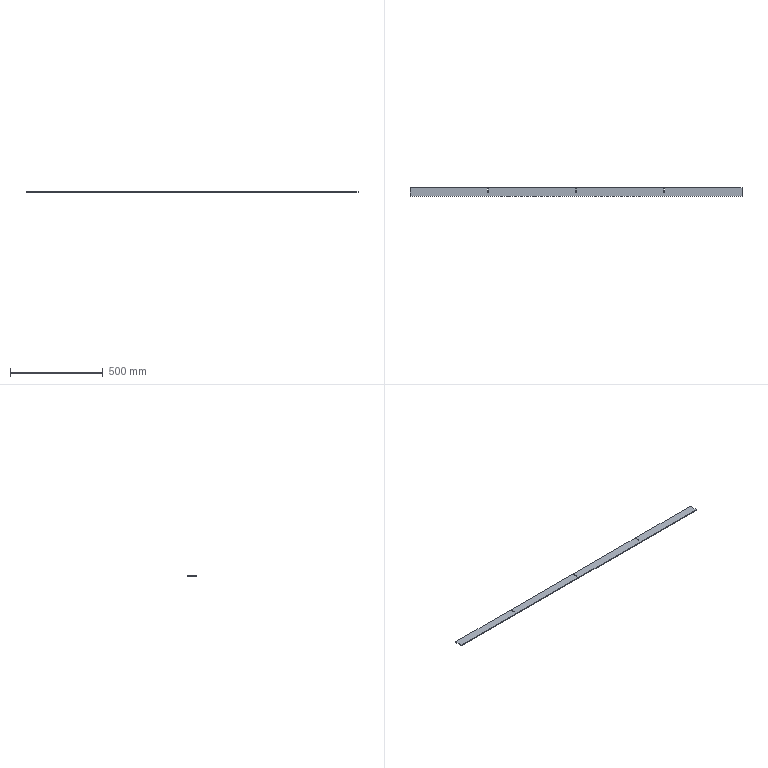Part | SolidWorks | features FlatPattern 1, SMBaseFlange 1, SheetMetal 1 | 1 solid | 18 faces | box 1790 x 45 x 4.5 mm | volume 360956 mm3 | plane 18
STEP:
#1=CARTESIAN_POINT('',(895.,-22.5,0.));
#2=VERTEX_POINT('',#1);
#3=CARTESIAN_POINT('',(895.,22.5,0.));
#4=VERTEX_POINT('',#3);
#5=CARTESIAN_POINT('',(895.,22.5,0.));
#6=DIRECTION('',(0.,1.,0.));
#7=VECTOR('',#6,1000.);
#8=LINE('',#5,#7);
#9=EDGE_CURVE('',#2,#4,#8,.T.);
#10=ORIENTED_EDGE('',*,*,#9,.F.);
#11=CARTESIAN_POINT('',(895.,-22.5,-4.5));
#12=VERTEX_POINT('',#11);
#13=CARTESIAN_POINT('',(895.,-22.5,-4.5));
#14=DIRECTION('',(0.,0.,1.));
#15=VECTOR('',#14,1000.);
#16=LINE('',#13,#15);
#17=EDGE_CURVE('',#12,#2,#16,.T.);
#18=ORIENTED_EDGE('',*,*,#17,.F.);
#19=CARTESIAN_POINT('',(895.,22.5,-4.5));
#20=VERTEX_POINT('',#19);
#21=CARTESIAN_POINT('',(895.,22.5,-4.5));
#22=DIRECTION('',(0.,1.,0.));
#23=VECTOR('',#22,1000.);
#24=LINE('',#21,#23);
#25=EDGE_CURVE('',#12,#20,#24,.T.);
#26=ORIENTED_EDGE('',*,*,#25,.T.);
#27=CARTESIAN_POINT('',(895.,22.5,-4.5));
#28=DIRECTION('',(0.,0.,1.));
#29=VECTOR('',#28,1000.);
#30=LINE('',#27,#29);
#31=EDGE_CURVE('',#20,#4,#30,.T.);
#32=ORIENTED_EDGE('',*,*,#31,.T.);
#33=EDGE_LOOP('',(#10,#18,#26,#32));
#34=FACE_OUTER_BOUND('',#33,.T.);
#35=CARTESIAN_POINT('',(895.,22.5,-4.5));
#36=DIRECTION('',(1.,0.,0.));
#37=DIRECTION('',(0.,0.,-1.));
#38=AXIS2_PLACEMENT_3D('',#35,#36,#37);
#39=PLANE('',#38);
#40=ADVANCED_FACE('',(#34),#39,.T.);
#41=CARTESIAN_POINT('',(-895.,-22.5,0.));
#42=VERTEX_POINT('',#41);
#43=CARTESIAN_POINT('',(-895.,-22.5,0.));
#44=DIRECTION('',(1.,0.,0.));
#45=VECTOR('',#44,1000.);
#46=LINE('',#43,#45);
#47=EDGE_CURVE('',#42,#2,#46,.T.);
#48=ORIENTED_EDGE('',*,*,#47,.F.);
#49=CARTESIAN_POINT('',(-895.,-22.5,-4.5));
#50=VERTEX_POINT('',#49);
#51=CARTESIAN_POINT('',(-895.,-22.5,-4.5));
#52=DIRECTION('',(0.,0.,1.));
#53=VECTOR('',#52,1000.);
#54=LINE('',#51,#53);
#55=EDGE_CURVE('',#50,#42,#54,.T.);
#56=ORIENTED_EDGE('',*,*,#55,.F.);
#57=CARTESIAN_POINT('',(-895.,-22.5,-4.5));
#58=DIRECTION('',(1.,0.,0.));
#59=VECTOR('',#58,1000.);
#60=LINE('',#57,#59);
#61=EDGE_CURVE('',#50,#12,#60,.T.);
#62=ORIENTED_EDGE('',*,*,#61,.T.);
#63=ORIENTED_EDGE('',*,*,#17,.T.);
#64=EDGE_LOOP('',(#48,#56,#62,#63));
#65=FACE_OUTER_BOUND('',#64,.T.);
#66=CARTESIAN_POINT('',(-895.,-22.5,-4.5));
#67=DIRECTION('',(0.,-1.,0.));
#68=DIRECTION('',(0.,0.,-1.));
#69=AXIS2_PLACEMENT_3D('',#66,#67,#68);
#70=PLANE('',#69);
#71=ADVANCED_FACE('',(#65),#70,.T.);
#72=CARTESIAN_POINT('',(-895.,22.5,0.));
#73=VERTEX_POINT('',#72);
#74=CARTESIAN_POINT('',(-895.,22.5,0.));
#75=DIRECTION('',(0.,-1.,0.));
#76=VECTOR('',#75,1000.);
#77=LINE('',#74,#76);
#78=EDGE_CURVE('',#73,#42,#77,.T.);
#79=ORIENTED_EDGE('',*,*,#78,.F.);
#80=CARTESIAN_POINT('',(-895.,22.5,-4.5));
#81=VERTEX_POINT('',#80);
#82=CARTESIAN_POINT('',(-895.,22.5,-4.5));
#83=DIRECTION('',(0.,0.,1.));
#84=VECTOR('',#83,1000.);
#85=LINE('',#82,#84);
#86=EDGE_CURVE('',#81,#73,#85,.T.);
#87=ORIENTED_EDGE('',*,*,#86,.F.);
#88=CARTESIAN_POINT('',(-895.,22.5,-4.5));
#89=DIRECTION('',(0.,-1.,0.));
#90=VECTOR('',#89,1000.);
#91=LINE('',#88,#90);
#92=EDGE_CURVE('',#81,#50,#91,.T.);
#93=ORIENTED_EDGE('',*,*,#92,.T.);
#94=ORIENTED_EDGE('',*,*,#55,.T.);
#95=EDGE_LOOP('',(#79,#87,#93,#94));
#96=FACE_OUTER_BOUND('',#95,.T.);
#97=CARTESIAN_POINT('',(-895.,22.5,-4.5));
#98=DIRECTION('',(-1.,0.,0.));
#99=DIRECTION('',(0.,0.,1.));
#100=AXIS2_PLACEMENT_3D('',#97,#98,#99);
#101=PLANE('',#100);
#102=ADVANCED_FACE('',(#96),#101,.T.);
#103=CARTESIAN_POINT('',(-477.25,22.5,0.));
#104=VERTEX_POINT('',#103);
#105=CARTESIAN_POINT('',(-895.,22.5,0.));
#106=DIRECTION('',(-1.,0.,0.));
#107=VECTOR('',#106,1000.);
#108=LINE('',#105,#107);
#109=EDGE_CURVE('',#104,#73,#108,.T.);
#110=ORIENTED_EDGE('',*,*,#109,.F.);
#111=CARTESIAN_POINT('',(-477.25,22.5,-4.5));
#112=VERTEX_POINT('',#111);
#113=CARTESIAN_POINT('',(-477.25,22.5,-4.5));
#114=DIRECTION('',(0.,0.,1.));
#115=VECTOR('',#114,1000.);
#116=LINE('',#113,#115);
#117=EDGE_CURVE('',#112,#104,#116,.T.);
#118=ORIENTED_EDGE('',*,*,#117,.F.);
#119=CARTESIAN_POINT('',(-895.,22.5,-4.5));
#120=DIRECTION('',(-1.,0.,0.));
#121=VECTOR('',#120,1000.);
#122=LINE('',#119,#121);
#123=EDGE_CURVE('',#112,#81,#122,.T.);
#124=ORIENTED_EDGE('',*,*,#123,.T.);
#125=ORIENTED_EDGE('',*,*,#86,.T.);
#126=EDGE_LOOP('',(#110,#118,#124,#125));
#127=FACE_OUTER_BOUND('',#126,.T.);
#128=CARTESIAN_POINT('',(-895.,22.5,-4.5));
#129=DIRECTION('',(0.,1.,0.));
#130=DIRECTION('',(-1.,0.,0.));
#131=AXIS2_PLACEMENT_3D('',#128,#129,#130);
#132=PLANE('',#131);
#133=ADVANCED_FACE('',(#127),#132,.T.);
#134=CARTESIAN_POINT('',(-477.25,-2.5,0.));
#135=VERTEX_POINT('',#134);
#136=CARTESIAN_POINT('',(-477.25,22.5,0.));
#137=DIRECTION('',(0.,1.,0.));
#138=VECTOR('',#137,1000.);
#139=LINE('',#136,#138);
#140=EDGE_CURVE('',#135,#104,#139,.T.);
#141=ORIENTED_EDGE('',*,*,#140,.F.);
#142=CARTESIAN_POINT('',(-477.25,-2.5,-4.5));
#143=VERTEX_POINT('',#142);
#144=CARTESIAN_POINT('',(-477.25,-2.5,-4.5));
#145=DIRECTION('',(0.,0.,1.));
#146=VECTOR('',#145,1000.);
#147=LINE('',#144,#146);
#148=EDGE_CURVE('',#143,#135,#147,.T.);
#149=ORIENTED_EDGE('',*,*,#148,.F.);
#150=CARTESIAN_POINT('',(-477.25,22.5,-4.5));
#151=DIRECTION('',(0.,1.,0.));
#152=VECTOR('',#151,1000.);
#153=LINE('',#150,#152);
#154=EDGE_CURVE('',#143,#112,#153,.T.);
#155=ORIENTED_EDGE('',*,*,#154,.T.);
#156=ORIENTED_EDGE('',*,*,#117,.T.);
#157=EDGE_LOOP('',(#141,#149,#155,#156));
#158=FACE_OUTER_BOUND('',#157,.T.);
#159=CARTESIAN_POINT('',(-477.25,22.5,-4.5));
#160=DIRECTION('',(1.,0.,0.));
#161=DIRECTION('',(0.,1.,0.));
#162=AXIS2_PLACEMENT_3D('',#159,#160,#161);
#163=PLANE('',#162);
#164=ADVANCED_FACE('',(#158),#163,.T.);
#165=CARTESIAN_POINT('',(-472.75,-2.5,0.));
#166=VERTEX_POINT('',#165);
#167=CARTESIAN_POINT('',(-477.25,-2.5,0.));
#168=DIRECTION('',(-1.,0.,0.));
#169=VECTOR('',#168,1000.);
#170=LINE('',#167,#169);
#171=EDGE_CURVE('',#166,#135,#170,.T.);
#172=ORIENTED_EDGE('',*,*,#171,.F.);
#173=CARTESIAN_POINT('',(-472.75,-2.5,-4.5));
#174=VERTEX_POINT('',#173);
#175=CARTESIAN_POINT('',(-472.75,-2.5,-4.5));
#176=DIRECTION('',(0.,0.,1.));
#177=VECTOR('',#176,1000.);
#178=LINE('',#175,#177);
#179=EDGE_CURVE('',#174,#166,#178,.T.);
#180=ORIENTED_EDGE('',*,*,#179,.F.);
#181=CARTESIAN_POINT('',(-477.25,-2.5,-4.5));
#182=DIRECTION('',(-1.,0.,0.));
#183=VECTOR('',#182,1000.);
#184=LINE('',#181,#183);
#185=EDGE_CURVE('',#174,#143,#184,.T.);
#186=ORIENTED_EDGE('',*,*,#185,.T.);
#187=ORIENTED_EDGE('',*,*,#148,.T.);
#188=EDGE_LOOP('',(#172,#180,#186,#187));
#189=FACE_OUTER_BOUND('',#188,.T.);
#190=CARTESIAN_POINT('',(-477.25,-2.5,-4.5));
#191=DIRECTION('',(0.,1.,0.));
#192=DIRECTION('',(0.,0.,1.));
#193=AXIS2_PLACEMENT_3D('',#190,#191,#192);
#194=PLANE('',#193);
#195=ADVANCED_FACE('',(#189),#194,.T.);
#196=CARTESIAN_POINT('',(-472.75,22.5,0.));
#197=VERTEX_POINT('',#196);
#198=CARTESIAN_POINT('',(-472.75,-2.5,0.));
#199=DIRECTION('',(0.,-1.,0.));
#200=VECTOR('',#199,1000.);
#201=LINE('',#198,#200);
#202=EDGE_CURVE('',#197,#166,#201,.T.);
#203=ORIENTED_EDGE('',*,*,#202,.F.);
#204=CARTESIAN_POINT('',(-472.75,22.5,-4.5));
#205=VERTEX_POINT('',#204);
#206=CARTESIAN_POINT('',(-472.75,22.5,-4.5));
#207=DIRECTION('',(0.,0.,1.));
#208=VECTOR('',#207,1000.);
#209=LINE('',#206,#208);
#210=EDGE_CURVE('',#205,#197,#209,.T.);
#211=ORIENTED_EDGE('',*,*,#210,.F.);
#212=CARTESIAN_POINT('',(-472.75,-2.5,-4.5));
#213=DIRECTION('',(0.,-1.,0.));
#214=VECTOR('',#213,1000.);
#215=LINE('',#212,#214);
#216=EDGE_CURVE('',#205,#174,#215,.T.);
#217=ORIENTED_EDGE('',*,*,#216,.T.);
#218=ORIENTED_EDGE('',*,*,#179,.T.);
#219=EDGE_LOOP('',(#203,#211,#217,#218));
#220=FACE_OUTER_BOUND('',#219,.T.);
#221=CARTESIAN_POINT('',(-472.75,-2.5,-4.5));
#222=DIRECTION('',(-1.,0.,0.));
#223=DIRECTION('',(0.,-1.,0.));
#224=AXIS2_PLACEMENT_3D('',#221,#222,#223);
#225=PLANE('',#224);
#226=ADVANCED_FACE('',(#220),#225,.T.);
#227=CARTESIAN_POINT('',(-2.25,22.5,0.));
#228=VERTEX_POINT('',#227);
#229=CARTESIAN_POINT('',(-472.75,22.5,0.));
#230=DIRECTION('',(-1.,0.,0.));
#231=VECTOR('',#230,1000.);
#232=LINE('',#229,#231);
#233=EDGE_CURVE('',#228,#197,#232,.T.);
#234=ORIENTED_EDGE('',*,*,#233,.F.);
#235=CARTESIAN_POINT('',(-2.25,22.5,-4.5));
#236=VERTEX_POINT('',#235);
#237=CARTESIAN_POINT('',(-2.25,22.5,-4.5));
#238=DIRECTION('',(0.,0.,1.));
#239=VECTOR('',#238,1000.);
#240=LINE('',#237,#239);
#241=EDGE_CURVE('',#236,#228,#240,.T.);
#242=ORIENTED_EDGE('',*,*,#241,.F.);
#243=CARTESIAN_POINT('',(-472.75,22.5,-4.5));
#244=DIRECTION('',(-1.,0.,0.));
#245=VECTOR('',#244,1000.);
#246=LINE('',#243,#245);
#247=EDGE_CURVE('',#236,#205,#246,.T.);
#248=ORIENTED_EDGE('',*,*,#247,.T.);
#249=ORIENTED_EDGE('',*,*,#210,.T.);
#250=EDGE_LOOP('',(#234,#242,#248,#249));
#251=FACE_OUTER_BOUND('',#250,.T.);
#252=CARTESIAN_POINT('',(-472.75,22.5,-4.5));
#253=DIRECTION('',(0.,1.,0.));
#254=DIRECTION('',(-1.,0.,0.));
#255=AXIS2_PLACEMENT_3D('',#252,#253,#254);
#256=PLANE('',#255);
#257=ADVANCED_FACE('',(#251),#256,.T.);
#258=CARTESIAN_POINT('',(-2.25,-2.5,0.));
#259=VERTEX_POINT('',#258);
#260=CARTESIAN_POINT('',(-2.25,22.5,0.));
#261=DIRECTION('',(0.,1.,0.));
#262=VECTOR('',#261,1000.);
#263=LINE('',#260,#262);
#264=EDGE_CURVE('',#259,#228,#263,.T.);
#265=ORIENTED_EDGE('',*,*,#264,.F.);
#266=CARTESIAN_POINT('',(-2.25,-2.5,-4.5));
#267=VERTEX_POINT('',#266);
#268=CARTESIAN_POINT('',(-2.25,-2.5,-4.5));
#269=DIRECTION('',(0.,0.,1.));
#270=VECTOR('',#269,1000.);
#271=LINE('',#268,#270);
#272=EDGE_CURVE('',#267,#259,#271,.T.);
#273=ORIENTED_EDGE('',*,*,#272,.F.);
#274=CARTESIAN_POINT('',(-2.25,22.5,-4.5));
#275=DIRECTION('',(0.,1.,0.));
#276=VECTOR('',#275,1000.);
#277=LINE('',#274,#276);
#278=EDGE_CURVE('',#267,#236,#277,.T.);
#279=ORIENTED_EDGE('',*,*,#278,.T.);
#280=ORIENTED_EDGE('',*,*,#241,.T.);
#281=EDGE_LOOP('',(#265,#273,#279,#280));
#282=FACE_OUTER_BOUND('',#281,.T.);
#283=CARTESIAN_POINT('',(-2.25,22.5,-4.5));
#284=DIRECTION('',(1.,0.,0.));
#285=DIRECTION('',(0.,1.,0.));
#286=AXIS2_PLACEMENT_3D('',#283,#284,#285);
#287=PLANE('',#286);
#288=ADVANCED_FACE('',(#282),#287,.T.);
#289=CARTESIAN_POINT('',(2.25,-2.5,0.));
#290=VERTEX_POINT('',#289);
#291=CARTESIAN_POINT('',(-2.25,-2.5,0.));
#292=DIRECTION('',(-1.,0.,0.));
#293=VECTOR('',#292,1000.);
#294=LINE('',#291,#293);
#295=EDGE_CURVE('',#290,#259,#294,.T.);
#296=ORIENTED_EDGE('',*,*,#295,.F.);
#297=CARTESIAN_POINT('',(2.25,-2.5,-4.5));
#298=VERTEX_POINT('',#297);
#299=CARTESIAN_POINT('',(2.25,-2.5,-4.5));
#300=DIRECTION('',(0.,0.,1.));
#301=VECTOR('',#300,1000.);
#302=LINE('',#299,#301);
#303=EDGE_CURVE('',#298,#290,#302,.T.);
#304=ORIENTED_EDGE('',*,*,#303,.F.);
#305=CARTESIAN_POINT('',(-2.25,-2.5,-4.5));
#306=DIRECTION('',(-1.,0.,0.));
#307=VECTOR('',#306,1000.);
#308=LINE('',#305,#307);
#309=EDGE_CURVE('',#298,#267,#308,.T.);
#310=ORIENTED_EDGE('',*,*,#309,.T.);
#311=ORIENTED_EDGE('',*,*,#272,.T.);
#312=EDGE_LOOP('',(#296,#304,#310,#311));
#313=FACE_OUTER_BOUND('',#312,.T.);
#314=CARTESIAN_POINT('',(-2.25,-2.5,-4.5));
#315=DIRECTION('',(0.,1.,0.));
#316=DIRECTION('',(0.,0.,1.));
#317=AXIS2_PLACEMENT_3D('',#314,#315,#316);
#318=PLANE('',#317);
#319=ADVANCED_FACE('',(#313),#318,.T.);
#320=CARTESIAN_POINT('',(2.25,22.5,0.));
#321=VERTEX_POINT('',#320);
#322=CARTESIAN_POINT('',(2.25,-2.5,0.));
#323=DIRECTION('',(0.,-1.,0.));
#324=VECTOR('',#323,1000.);
#325=LINE('',#322,#324);
#326=EDGE_CURVE('',#321,#290,#325,.T.);
#327=ORIENTED_EDGE('',*,*,#326,.F.);
#328=CARTESIAN_POINT('',(2.25,22.5,-4.5));
#329=VERTEX_POINT('',#328);
#330=CARTESIAN_POINT('',(2.25,22.5,-4.5));
#331=DIRECTION('',(0.,0.,1.));
#332=VECTOR('',#331,1000.);
#333=LINE('',#330,#332);
#334=EDGE_CURVE('',#329,#321,#333,.T.);
#335=ORIENTED_EDGE('',*,*,#334,.F.);
#336=CARTESIAN_POINT('',(2.25,-2.5,-4.5));
#337=DIRECTION('',(0.,-1.,0.));
#338=VECTOR('',#337,1000.);
#339=LINE('',#336,#338);
#340=EDGE_CURVE('',#329,#298,#339,.T.);
#341=ORIENTED_EDGE('',*,*,#340,.T.);
#342=ORIENTED_EDGE('',*,*,#303,.T.);
#343=EDGE_LOOP('',(#327,#335,#341,#342));
#344=FACE_OUTER_BOUND('',#343,.T.);
#345=CARTESIAN_POINT('',(2.25,-2.5,-4.5));
#346=DIRECTION('',(-1.,0.,0.));
#347=DIRECTION('',(0.,-1.,0.));
#348=AXIS2_PLACEMENT_3D('',#345,#346,#347);
#349=PLANE('',#348);
#350=ADVANCED_FACE('',(#344),#349,.T.);
#351=CARTESIAN_POINT('',(472.75,22.5,0.));
#352=VERTEX_POINT('',#351);
#353=CARTESIAN_POINT('',(2.25,22.5,0.));
#354=DIRECTION('',(-1.,0.,0.));
#355=VECTOR('',#354,1000.);
#356=LINE('',#353,#355);
#357=EDGE_CURVE('',#352,#321,#356,.T.);
#358=ORIENTED_EDGE('',*,*,#357,.F.);
#359=CARTESIAN_POINT('',(472.75,22.5,-4.5));
#360=VERTEX_POINT('',#359);
#361=CARTESIAN_POINT('',(472.75,22.5,-4.5));
#362=DIRECTION('',(0.,0.,1.));
#363=VECTOR('',#362,1000.);
#364=LINE('',#361,#363);
#365=EDGE_CURVE('',#360,#352,#364,.T.);
#366=ORIENTED_EDGE('',*,*,#365,.F.);
#367=CARTESIAN_POINT('',(2.25,22.5,-4.5));
#368=DIRECTION('',(-1.,0.,0.));
#369=VECTOR('',#368,1000.);
#370=LINE('',#367,#369);
#371=EDGE_CURVE('',#360,#329,#370,.T.);
#372=ORIENTED_EDGE('',*,*,#371,.T.);
#373=ORIENTED_EDGE('',*,*,#334,.T.);
#374=EDGE_LOOP('',(#358,#366,#372,#373));
#375=FACE_OUTER_BOUND('',#374,.T.);
#376=CARTESIAN_POINT('',(2.25,22.5,-4.5));
#377=DIRECTION('',(0.,1.,0.));
#378=DIRECTION('',(-1.,0.,0.));
#379=AXIS2_PLACEMENT_3D('',#376,#377,#378);
#380=PLANE('',#379);
#381=ADVANCED_FACE('',(#375),#380,.T.);
#382=CARTESIAN_POINT('',(472.75,-2.5,0.));
#383=VERTEX_POINT('',#382);
#384=CARTESIAN_POINT('',(472.75,22.5,0.));
#385=DIRECTION('',(0.,1.,0.));
#386=VECTOR('',#385,1000.);
#387=LINE('',#384,#386);
#388=EDGE_CURVE('',#383,#352,#387,.T.);
#389=ORIENTED_EDGE('',*,*,#388,.F.);
#390=CARTESIAN_POINT('',(472.75,-2.5,-4.5));
#391=VERTEX_POINT('',#390);
#392=CARTESIAN_POINT('',(472.75,-2.5,-4.5));
#393=DIRECTION('',(0.,0.,1.));
#394=VECTOR('',#393,1000.);
#395=LINE('',#392,#394);
#396=EDGE_CURVE('',#391,#383,#395,.T.);
#397=ORIENTED_EDGE('',*,*,#396,.F.);
#398=CARTESIAN_POINT('',(472.75,22.5,-4.5));
#399=DIRECTION('',(0.,1.,0.));
#400=VECTOR('',#399,1000.);
#401=LINE('',#398,#400);
#402=EDGE_CURVE('',#391,#360,#401,.T.);
#403=ORIENTED_EDGE('',*,*,#402,.T.);
#404=ORIENTED_EDGE('',*,*,#365,.T.);
#405=EDGE_LOOP('',(#389,#397,#403,#404));
#406=FACE_OUTER_BOUND('',#405,.T.);
#407=CARTESIAN_POINT('',(472.75,22.5,-4.5));
#408=DIRECTION('',(1.,0.,0.));
#409=DIRECTION('',(0.,1.,0.));
#410=AXIS2_PLACEMENT_3D('',#407,#408,#409);
#411=PLANE('',#410);
#412=ADVANCED_FACE('',(#406),#411,.T.);
#413=CARTESIAN_POINT('',(477.25,-2.5,0.));
#414=VERTEX_POINT('',#413);
#415=CARTESIAN_POINT('',(472.75,-2.5,0.));
#416=DIRECTION('',(-1.,0.,0.));
#417=VECTOR('',#416,1000.);
#418=LINE('',#415,#417);
#419=EDGE_CURVE('',#414,#383,#418,.T.);
#420=ORIENTED_EDGE('',*,*,#419,.F.);
#421=CARTESIAN_POINT('',(477.25,-2.5,-4.5));
#422=VERTEX_POINT('',#421);
#423=CARTESIAN_POINT('',(477.25,-2.5,-4.5));
#424=DIRECTION('',(0.,0.,1.));
#425=VECTOR('',#424,1000.);
#426=LINE('',#423,#425);
#427=EDGE_CURVE('',#422,#414,#426,.T.);
#428=ORIENTED_EDGE('',*,*,#427,.F.);
#429=CARTESIAN_POINT('',(472.75,-2.5,-4.5));
#430=DIRECTION('',(-1.,0.,0.));
#431=VECTOR('',#430,1000.);
#432=LINE('',#429,#431);
#433=EDGE_CURVE('',#422,#391,#432,.T.);
#434=ORIENTED_EDGE('',*,*,#433,.T.);
#435=ORIENTED_EDGE('',*,*,#396,.T.);
#436=EDGE_LOOP('',(#420,#428,#434,#435));
#437=FACE_OUTER_BOUND('',#436,.T.);
#438=CARTESIAN_POINT('',(472.75,-2.5,-4.5));
#439=DIRECTION('',(0.,1.,0.));
#440=DIRECTION('',(0.,0.,1.));
#441=AXIS2_PLACEMENT_3D('',#438,#439,#440);
#442=PLANE('',#441);
#443=ADVANCED_FACE('',(#437),#442,.T.);
#444=CARTESIAN_POINT('',(477.25,22.5,0.));
#445=VERTEX_POINT('',#444);
#446=CARTESIAN_POINT('',(477.25,-2.5,0.));
#447=DIRECTION('',(0.,-1.,0.));
#448=VECTOR('',#447,1000.);
#449=LINE('',#446,#448);
#450=EDGE_CURVE('',#445,#414,#449,.T.);
#451=ORIENTED_EDGE('',*,*,#450,.F.);
#452=CARTESIAN_POINT('',(477.25,22.5,-4.5));
#453=VERTEX_POINT('',#452);
#454=CARTESIAN_POINT('',(477.25,22.5,-4.5));
#455=DIRECTION('',(0.,0.,1.));
#456=VECTOR('',#455,1000.);
#457=LINE('',#454,#456);
#458=EDGE_CURVE('',#453,#445,#457,.T.);
#459=ORIENTED_EDGE('',*,*,#458,.F.);
#460=CARTESIAN_POINT('',(477.25,-2.5,-4.5));
#461=DIRECTION('',(0.,-1.,0.));
#462=VECTOR('',#461,1000.);
#463=LINE('',#460,#462);
#464=EDGE_CURVE('',#453,#422,#463,.T.);
#465=ORIENTED_EDGE('',*,*,#464,.T.);
#466=ORIENTED_EDGE('',*,*,#427,.T.);
#467=EDGE_LOOP('',(#451,#459,#465,#466));
#468=FACE_OUTER_BOUND('',#467,.T.);
#469=CARTESIAN_POINT('',(477.25,-2.5,-4.5));
#470=DIRECTION('',(-1.,0.,0.));
#471=DIRECTION('',(0.,-1.,0.));
#472=AXIS2_PLACEMENT_3D('',#469,#470,#471);
#473=PLANE('',#472);
#474=ADVANCED_FACE('',(#468),#473,.T.);
#475=CARTESIAN_POINT('',(477.25,22.5,0.));
#476=DIRECTION('',(-1.,0.,0.));
#477=VECTOR('',#476,1000.);
#478=LINE('',#475,#477);
#479=EDGE_CURVE('',#4,#445,#478,.T.);
#480=ORIENTED_EDGE('',*,*,#479,.F.);
#481=ORIENTED_EDGE('',*,*,#31,.F.);
#482=CARTESIAN_POINT('',(477.25,22.5,-4.5));
#483=DIRECTION('',(-1.,0.,0.));
#484=VECTOR('',#483,1000.);
#485=LINE('',#482,#484);
#486=EDGE_CURVE('',#20,#453,#485,.T.);
#487=ORIENTED_EDGE('',*,*,#486,.T.);
#488=ORIENTED_EDGE('',*,*,#458,.T.);
#489=EDGE_LOOP('',(#480,#481,#487,#488));
#490=FACE_OUTER_BOUND('',#489,.T.);
#491=CARTESIAN_POINT('',(477.25,22.5,-4.5));
#492=DIRECTION('',(0.,1.,0.));
#493=DIRECTION('',(-1.,0.,0.));
#494=AXIS2_PLACEMENT_3D('',#491,#492,#493);
#495=PLANE('',#494);
#496=ADVANCED_FACE('',(#490),#495,.T.);
#497=ORIENTED_EDGE('',*,*,#25,.F.);
#498=ORIENTED_EDGE('',*,*,#61,.F.);
#499=ORIENTED_EDGE('',*,*,#92,.F.);
#500=ORIENTED_EDGE('',*,*,#123,.F.);
#501=ORIENTED_EDGE('',*,*,#154,.F.);
#502=ORIENTED_EDGE('',*,*,#185,.F.);
#503=ORIENTED_EDGE('',*,*,#216,.F.);
#504=ORIENTED_EDGE('',*,*,#247,.F.);
#505=ORIENTED_EDGE('',*,*,#278,.F.);
#506=ORIENTED_EDGE('',*,*,#309,.F.);
#507=ORIENTED_EDGE('',*,*,#340,.F.);
#508=ORIENTED_EDGE('',*,*,#371,.F.);
#509=ORIENTED_EDGE('',*,*,#402,.F.);
#510=ORIENTED_EDGE('',*,*,#433,.F.);
#511=ORIENTED_EDGE('',*,*,#464,.F.);
#512=ORIENTED_EDGE('',*,*,#486,.F.);
#513=EDGE_LOOP('',(#497,#498,#499,#500,#501,#502,#503,#504,#505,#506,#507,#508,#509,#510,#511,#512));
#514=FACE_OUTER_BOUND('',#513,.T.);
#515=CARTESIAN_POINT('',(0.,0.,-4.5));
#516=DIRECTION('',(0.,0.,1.));
#517=DIRECTION('',(1.,0.,0.));
#518=AXIS2_PLACEMENT_3D('',#515,#516,#517);
#519=PLANE('',#518);
#520=ADVANCED_FACE('',(#514),#519,.F.);
#521=ORIENTED_EDGE('',*,*,#9,.T.);
#522=ORIENTED_EDGE('',*,*,#479,.T.);
#523=ORIENTED_EDGE('',*,*,#450,.T.);
#524=ORIENTED_EDGE('',*,*,#419,.T.);
#525=ORIENTED_EDGE('',*,*,#388,.T.);
#526=ORIENTED_EDGE('',*,*,#357,.T.);
#527=ORIENTED_EDGE('',*,*,#326,.T.);
#528=ORIENTED_EDGE('',*,*,#295,.T.);
#529=ORIENTED_EDGE('',*,*,#264,.T.);
#530=ORIENTED_EDGE('',*,*,#233,.T.);
#531=ORIENTED_EDGE('',*,*,#202,.T.);
#532=ORIENTED_EDGE('',*,*,#171,.T.);
#533=ORIENTED_EDGE('',*,*,#140,.T.);
#534=ORIENTED_EDGE('',*,*,#109,.T.);
#535=ORIENTED_EDGE('',*,*,#78,.T.);
#536=ORIENTED_EDGE('',*,*,#47,.T.);
#537=EDGE_LOOP('',(#521,#522,#523,#524,#525,#526,#527,#528,#529,#530,#531,#532,#533,#534,#535,#536));
#538=FACE_OUTER_BOUND('',#537,.T.);
#539=CARTESIAN_POINT('',(0.,0.,0.));
#540=DIRECTION('',(0.,0.,1.));
#541=DIRECTION('',(1.,0.,0.));
#542=AXIS2_PLACEMENT_3D('',#539,#540,#541);
#543=PLANE('',#542);
#544=ADVANCED_FACE('',(#538),#543,.T.);
#545=CLOSED_SHELL('',(#40,#71,#102,#133,#164,#195,#226,#257,#288,#319,#350,#381,#412,#443,#474,#496,#520,#544));
#546=MANIFOLD_SOLID_BREP('',#545);
#547=CARTESIAN_POINT('',(0.,0.,0.));
#548=DIRECTION('',(0.,0.,1.));
#549=DIRECTION('',(1.,0.,0.));
#550=AXIS2_PLACEMENT_3D('',#547,#548,#549);
#551=(LENGTH_UNIT()NAMED_UNIT(*)SI_UNIT(.MILLI.,.METRE.));
#552=UNCERTAINTY_MEASURE_WITH_UNIT(LENGTH_MEASURE(0.00001),#551,'','');
#553=(NAMED_UNIT(*)PLANE_ANGLE_UNIT()SI_UNIT($,.RADIAN.));
#554=(NAMED_UNIT(*)SI_UNIT($,.STERADIAN.)SOLID_ANGLE_UNIT());
#555=(GEOMETRIC_REPRESENTATION_CONTEXT(3)GLOBAL_UNCERTAINTY_ASSIGNED_CONTEXT((#552))GLOBAL_UNIT_ASSIGNED_CONTEXT((#551,#553,#554))REPRESENTATION_CONTEXT('',''));
#556=ADVANCED_BREP_SHAPE_REPRESENTATION('',(#546,#550),#555);